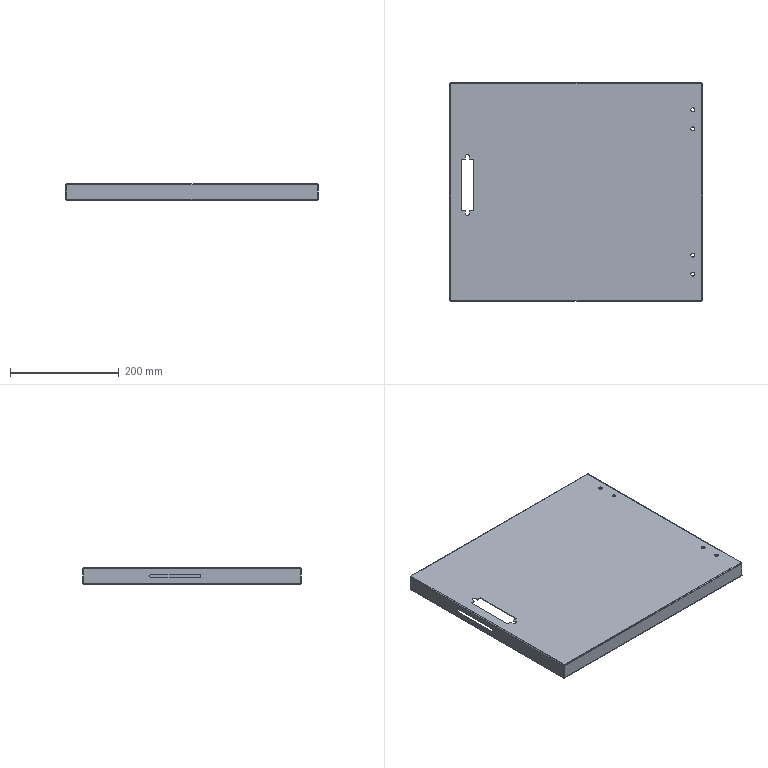Part | 1 solid | 95 faces | box 463 x 402 x 30 mm | volume 298410 mm3 | plane 50 | cylinder 29 | spline 16 | commonest cylinder face diameters 7 x13 1.473 x8 3.873 x8